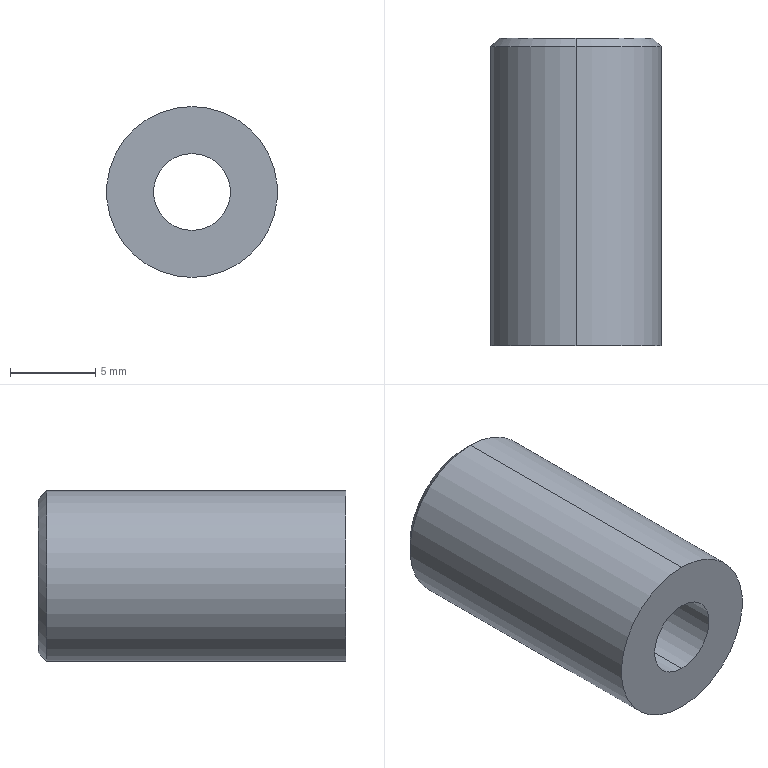Part | SolidWorks | features Chamfer 1, Extrusion 1, HoleWzd 1 | 1 solid | 11 faces | box 10 x 18 x 10 mm | volume 965.582 mm3 | cylinder 6 | plane 3 | cone 2 | commonest cylinder face diameters 4.5 x2 8 x2 10 x2
STEP:
#1=CARTESIAN_POINT('',(0.,18.,4.5));
#2=VERTEX_POINT('',#1);
#3=CARTESIAN_POINT('',(0.,18.,-4.5));
#4=VERTEX_POINT('',#3);
#5=CARTESIAN_POINT('',(0.,18.,0.));
#6=DIRECTION('',(0.,1.,0.));
#7=DIRECTION('',(0.,0.,1.));
#8=AXIS2_PLACEMENT_3D('',#5,#6,#7);
#9=CIRCLE('',#8,4.5);
#10=EDGE_CURVE('',#2,#4,#9,.T.);
#11=ORIENTED_EDGE('',*,*,#10,.F.);
#12=CARTESIAN_POINT('',(0.,17.5,5.));
#13=VERTEX_POINT('',#12);
#14=CARTESIAN_POINT('',(0.,18.,4.5));
#15=DIRECTION('',(0.,-0.7071,0.7071));
#16=VECTOR('',#15,1000.);
#17=LINE('',#14,#16);
#18=EDGE_CURVE('',#2,#13,#17,.T.);
#19=ORIENTED_EDGE('',*,*,#18,.T.);
#20=CARTESIAN_POINT('',(0.,17.5,-5.));
#21=VERTEX_POINT('',#20);
#22=CARTESIAN_POINT('',(0.,17.5,0.));
#23=DIRECTION('',(0.,-1.,0.));
#24=DIRECTION('',(0.,0.,1.));
#25=AXIS2_PLACEMENT_3D('',#22,#23,#24);
#26=CIRCLE('',#25,5.);
#27=EDGE_CURVE('',#21,#13,#26,.T.);
#28=ORIENTED_EDGE('',*,*,#27,.F.);
#29=CARTESIAN_POINT('',(0.,18.,-4.5));
#30=DIRECTION('',(0.,-0.7071,-0.7071));
#31=VECTOR('',#30,1000.);
#32=LINE('',#29,#31);
#33=EDGE_CURVE('',#4,#21,#32,.T.);
#34=ORIENTED_EDGE('',*,*,#33,.F.);
#35=EDGE_LOOP('',(#11,#19,#28,#34));
#36=FACE_OUTER_BOUND('',#35,.T.);
#37=CARTESIAN_POINT('',(0.,18.,0.));
#38=DIRECTION('',(0.,-1.,0.));
#39=DIRECTION('',(0.,0.,-1.));
#40=AXIS2_PLACEMENT_3D('',#37,#38,#39);
#41=CONICAL_SURFACE('',#40,4.5,0.7854);
#42=ADVANCED_FACE('',(#36),#41,.T.);
#43=CARTESIAN_POINT('',(0.,13.4,-4.));
#44=VERTEX_POINT('',#43);
#45=CARTESIAN_POINT('',(0.,13.4,4.));
#46=VERTEX_POINT('',#45);
#47=CARTESIAN_POINT('',(0.,13.4,0.));
#48=DIRECTION('',(0.,1.,0.));
#49=DIRECTION('',(0.,0.,1.));
#50=AXIS2_PLACEMENT_3D('',#47,#48,#49);
#51=CIRCLE('',#50,4.);
#52=EDGE_CURVE('',#44,#46,#51,.T.);
#53=ORIENTED_EDGE('',*,*,#52,.F.);
#54=CARTESIAN_POINT('',(0.,18.,-4.));
#55=VERTEX_POINT('',#54);
#56=CARTESIAN_POINT('',(0.,18.,-4.));
#57=DIRECTION('',(0.,1.,0.));
#58=VECTOR('',#57,1000.);
#59=LINE('',#56,#58);
#60=EDGE_CURVE('',#44,#55,#59,.T.);
#61=ORIENTED_EDGE('',*,*,#60,.T.);
#62=CARTESIAN_POINT('',(0.,18.,4.));
#63=VERTEX_POINT('',#62);
#64=CARTESIAN_POINT('',(0.,18.,0.));
#65=DIRECTION('',(0.,1.,0.));
#66=DIRECTION('',(0.,0.,1.));
#67=AXIS2_PLACEMENT_3D('',#64,#65,#66);
#68=CIRCLE('',#67,4.);
#69=EDGE_CURVE('',#55,#63,#68,.T.);
#70=ORIENTED_EDGE('',*,*,#69,.T.);
#71=CARTESIAN_POINT('',(0.,18.,4.));
#72=DIRECTION('',(0.,1.,0.));
#73=VECTOR('',#72,1000.);
#74=LINE('',#71,#73);
#75=EDGE_CURVE('',#46,#63,#74,.T.);
#76=ORIENTED_EDGE('',*,*,#75,.F.);
#77=EDGE_LOOP('',(#53,#61,#70,#76));
#78=FACE_OUTER_BOUND('',#77,.T.);
#79=CARTESIAN_POINT('',(0.,18.,0.));
#80=DIRECTION('',(0.,1.,0.));
#81=DIRECTION('',(0.,0.,1.));
#82=AXIS2_PLACEMENT_3D('',#79,#80,#81);
#83=CYLINDRICAL_SURFACE('',#82,4.);
#84=ADVANCED_FACE('',(#78),#83,.F.);
#85=CARTESIAN_POINT('',(0.,0.,-2.25));
#86=VERTEX_POINT('',#85);
#87=CARTESIAN_POINT('',(0.,0.,2.25));
#88=VERTEX_POINT('',#87);
#89=CARTESIAN_POINT('',(0.,0.,0.));
#90=DIRECTION('',(0.,1.,0.));
#91=DIRECTION('',(0.,0.,1.));
#92=AXIS2_PLACEMENT_3D('',#89,#90,#91);
#93=CIRCLE('',#92,2.25);
#94=EDGE_CURVE('',#86,#88,#93,.T.);
#95=ORIENTED_EDGE('',*,*,#94,.F.);
#96=CARTESIAN_POINT('',(0.,13.4,-2.25));
#97=VERTEX_POINT('',#96);
#98=CARTESIAN_POINT('',(0.,18.,-2.25));
#99=DIRECTION('',(0.,1.,0.));
#100=VECTOR('',#99,1000.);
#101=LINE('',#98,#100);
#102=EDGE_CURVE('',#86,#97,#101,.T.);
#103=ORIENTED_EDGE('',*,*,#102,.T.);
#104=CARTESIAN_POINT('',(0.,13.4,2.25));
#105=VERTEX_POINT('',#104);
#106=CARTESIAN_POINT('',(0.,13.4,0.));
#107=DIRECTION('',(0.,1.,0.));
#108=DIRECTION('',(0.,0.,1.));
#109=AXIS2_PLACEMENT_3D('',#106,#107,#108);
#110=CIRCLE('',#109,2.25);
#111=EDGE_CURVE('',#97,#105,#110,.T.);
#112=ORIENTED_EDGE('',*,*,#111,.T.);
#113=CARTESIAN_POINT('',(0.,18.,2.25));
#114=DIRECTION('',(0.,1.,0.));
#115=VECTOR('',#114,1000.);
#116=LINE('',#113,#115);
#117=EDGE_CURVE('',#88,#105,#116,.T.);
#118=ORIENTED_EDGE('',*,*,#117,.F.);
#119=EDGE_LOOP('',(#95,#103,#112,#118));
#120=FACE_OUTER_BOUND('',#119,.T.);
#121=CARTESIAN_POINT('',(0.,18.,0.));
#122=DIRECTION('',(0.,1.,0.));
#123=DIRECTION('',(0.,0.,1.));
#124=AXIS2_PLACEMENT_3D('',#121,#122,#123);
#125=CYLINDRICAL_SURFACE('',#124,2.25);
#126=ADVANCED_FACE('',(#120),#125,.F.);
#127=ORIENTED_EDGE('',*,*,#27,.T.);
#128=CARTESIAN_POINT('',(0.,0.,5.));
#129=VERTEX_POINT('',#128);
#130=CARTESIAN_POINT('',(0.,18.,5.));
#131=DIRECTION('',(0.,-1.,0.));
#132=VECTOR('',#131,1000.);
#133=LINE('',#130,#132);
#134=EDGE_CURVE('',#13,#129,#133,.T.);
#135=ORIENTED_EDGE('',*,*,#134,.T.);
#136=CARTESIAN_POINT('',(0.,0.,-5.));
#137=VERTEX_POINT('',#136);
#138=CARTESIAN_POINT('',(0.,0.,0.));
#139=DIRECTION('',(0.,1.,0.));
#140=DIRECTION('',(0.,0.,1.));
#141=AXIS2_PLACEMENT_3D('',#138,#139,#140);
#142=CIRCLE('',#141,5.);
#143=EDGE_CURVE('',#129,#137,#142,.T.);
#144=ORIENTED_EDGE('',*,*,#143,.T.);
#145=CARTESIAN_POINT('',(0.,18.,-5.));
#146=DIRECTION('',(0.,-1.,0.));
#147=VECTOR('',#146,1000.);
#148=LINE('',#145,#147);
#149=EDGE_CURVE('',#21,#137,#148,.T.);
#150=ORIENTED_EDGE('',*,*,#149,.F.);
#151=EDGE_LOOP('',(#127,#135,#144,#150));
#152=FACE_OUTER_BOUND('',#151,.T.);
#153=CARTESIAN_POINT('',(0.,18.,0.));
#154=DIRECTION('',(0.,-1.,0.));
#155=DIRECTION('',(0.,0.,-1.));
#156=AXIS2_PLACEMENT_3D('',#153,#154,#155);
#157=CYLINDRICAL_SURFACE('',#156,5.);
#158=ADVANCED_FACE('',(#152),#157,.T.);
#159=ORIENTED_EDGE('',*,*,#134,.F.);
#160=CARTESIAN_POINT('',(0.,17.5,0.));
#161=DIRECTION('',(0.,-1.,0.));
#162=DIRECTION('',(0.,0.,1.));
#163=AXIS2_PLACEMENT_3D('',#160,#161,#162);
#164=CIRCLE('',#163,5.);
#165=EDGE_CURVE('',#13,#21,#164,.T.);
#166=ORIENTED_EDGE('',*,*,#165,.T.);
#167=ORIENTED_EDGE('',*,*,#149,.T.);
#168=CARTESIAN_POINT('',(0.,0.,0.));
#169=DIRECTION('',(0.,1.,0.));
#170=DIRECTION('',(0.,0.,1.));
#171=AXIS2_PLACEMENT_3D('',#168,#169,#170);
#172=CIRCLE('',#171,5.);
#173=EDGE_CURVE('',#137,#129,#172,.T.);
#174=ORIENTED_EDGE('',*,*,#173,.T.);
#175=EDGE_LOOP('',(#159,#166,#167,#174));
#176=FACE_OUTER_BOUND('',#175,.T.);
#177=CARTESIAN_POINT('',(0.,18.,0.));
#178=DIRECTION('',(0.,-1.,0.));
#179=DIRECTION('',(0.,0.,-1.));
#180=AXIS2_PLACEMENT_3D('',#177,#178,#179);
#181=CYLINDRICAL_SURFACE('',#180,5.);
#182=ADVANCED_FACE('',(#176),#181,.T.);
#183=CARTESIAN_POINT('',(0.,18.,0.));
#184=DIRECTION('',(0.,1.,0.));
#185=DIRECTION('',(0.,0.,1.));
#186=AXIS2_PLACEMENT_3D('',#183,#184,#185);
#187=CIRCLE('',#186,4.5);
#188=EDGE_CURVE('',#4,#2,#187,.T.);
#189=ORIENTED_EDGE('',*,*,#188,.T.);
#190=ORIENTED_EDGE('',*,*,#10,.T.);
#191=EDGE_LOOP('',(#189,#190));
#192=FACE_OUTER_BOUND('',#191,.T.);
#193=CARTESIAN_POINT('',(0.,18.,0.));
#194=DIRECTION('',(0.,1.,0.));
#195=DIRECTION('',(0.,0.,1.));
#196=AXIS2_PLACEMENT_3D('',#193,#194,#195);
#197=CIRCLE('',#196,4.);
#198=EDGE_CURVE('',#63,#55,#197,.T.);
#199=ORIENTED_EDGE('',*,*,#198,.F.);
#200=ORIENTED_EDGE('',*,*,#69,.F.);
#201=EDGE_LOOP('',(#199,#200));
#202=FACE_BOUND('',#201,.T.);
#203=CARTESIAN_POINT('',(0.,18.,0.));
#204=DIRECTION('',(0.,1.,0.));
#205=DIRECTION('',(0.,0.,1.));
#206=AXIS2_PLACEMENT_3D('',#203,#204,#205);
#207=PLANE('',#206);
#208=ADVANCED_FACE('',(#192,#202),#207,.T.);
#209=CARTESIAN_POINT('',(0.,0.,0.));
#210=DIRECTION('',(0.,1.,0.));
#211=DIRECTION('',(0.,0.,1.));
#212=AXIS2_PLACEMENT_3D('',#209,#210,#211);
#213=CIRCLE('',#212,2.25);
#214=EDGE_CURVE('',#88,#86,#213,.T.);
#215=ORIENTED_EDGE('',*,*,#214,.T.);
#216=ORIENTED_EDGE('',*,*,#94,.T.);
#217=EDGE_LOOP('',(#215,#216));
#218=FACE_BOUND('',#217,.T.);
#219=ORIENTED_EDGE('',*,*,#173,.F.);
#220=ORIENTED_EDGE('',*,*,#143,.F.);
#221=EDGE_LOOP('',(#219,#220));
#222=FACE_OUTER_BOUND('',#221,.T.);
#223=CARTESIAN_POINT('',(0.,0.,0.));
#224=DIRECTION('',(0.,1.,0.));
#225=DIRECTION('',(0.,0.,1.));
#226=AXIS2_PLACEMENT_3D('',#223,#224,#225);
#227=PLANE('',#226);
#228=ADVANCED_FACE('',(#218,#222),#227,.F.);
#229=ORIENTED_EDGE('',*,*,#102,.F.);
#230=ORIENTED_EDGE('',*,*,#214,.F.);
#231=ORIENTED_EDGE('',*,*,#117,.T.);
#232=CARTESIAN_POINT('',(0.,13.4,0.));
#233=DIRECTION('',(0.,1.,0.));
#234=DIRECTION('',(0.,0.,1.));
#235=AXIS2_PLACEMENT_3D('',#232,#233,#234);
#236=CIRCLE('',#235,2.25);
#237=EDGE_CURVE('',#105,#97,#236,.T.);
#238=ORIENTED_EDGE('',*,*,#237,.T.);
#239=EDGE_LOOP('',(#229,#230,#231,#238));
#240=FACE_OUTER_BOUND('',#239,.T.);
#241=CARTESIAN_POINT('',(0.,18.,0.));
#242=DIRECTION('',(0.,1.,0.));
#243=DIRECTION('',(0.,0.,1.));
#244=AXIS2_PLACEMENT_3D('',#241,#242,#243);
#245=CYLINDRICAL_SURFACE('',#244,2.25);
#246=ADVANCED_FACE('',(#240),#245,.F.);
#247=ORIENTED_EDGE('',*,*,#237,.F.);
#248=ORIENTED_EDGE('',*,*,#111,.F.);
#249=EDGE_LOOP('',(#247,#248));
#250=FACE_BOUND('',#249,.T.);
#251=CARTESIAN_POINT('',(0.,13.4,0.));
#252=DIRECTION('',(0.,1.,0.));
#253=DIRECTION('',(0.,0.,1.));
#254=AXIS2_PLACEMENT_3D('',#251,#252,#253);
#255=CIRCLE('',#254,4.);
#256=EDGE_CURVE('',#46,#44,#255,.T.);
#257=ORIENTED_EDGE('',*,*,#256,.T.);
#258=ORIENTED_EDGE('',*,*,#52,.T.);
#259=EDGE_LOOP('',(#257,#258));
#260=FACE_OUTER_BOUND('',#259,.T.);
#261=CARTESIAN_POINT('',(2.25,13.4,0.));
#262=DIRECTION('',(0.,-1.,0.));
#263=DIRECTION('',(0.,0.,-1.));
#264=AXIS2_PLACEMENT_3D('',#261,#262,#263);
#265=PLANE('',#264);
#266=ADVANCED_FACE('',(#250,#260),#265,.F.);
#267=ORIENTED_EDGE('',*,*,#60,.F.);
#268=ORIENTED_EDGE('',*,*,#256,.F.);
#269=ORIENTED_EDGE('',*,*,#75,.T.);
#270=ORIENTED_EDGE('',*,*,#198,.T.);
#271=EDGE_LOOP('',(#267,#268,#269,#270));
#272=FACE_OUTER_BOUND('',#271,.T.);
#273=CARTESIAN_POINT('',(0.,18.,0.));
#274=DIRECTION('',(0.,1.,0.));
#275=DIRECTION('',(0.,0.,1.));
#276=AXIS2_PLACEMENT_3D('',#273,#274,#275);
#277=CYLINDRICAL_SURFACE('',#276,4.);
#278=ADVANCED_FACE('',(#272),#277,.F.);
#279=ORIENTED_EDGE('',*,*,#18,.F.);
#280=ORIENTED_EDGE('',*,*,#188,.F.);
#281=ORIENTED_EDGE('',*,*,#33,.T.);
#282=ORIENTED_EDGE('',*,*,#165,.F.);
#283=EDGE_LOOP('',(#279,#280,#281,#282));
#284=FACE_OUTER_BOUND('',#283,.T.);
#285=CARTESIAN_POINT('',(0.,18.,0.));
#286=DIRECTION('',(0.,-1.,0.));
#287=DIRECTION('',(0.,0.,-1.));
#288=AXIS2_PLACEMENT_3D('',#285,#286,#287);
#289=CONICAL_SURFACE('',#288,4.5,0.7854);
#290=ADVANCED_FACE('',(#284),#289,.T.);
#291=CLOSED_SHELL('',(#42,#84,#126,#158,#182,#208,#228,#246,#266,#278,#290));
#292=MANIFOLD_SOLID_BREP('',#291);
#293=CARTESIAN_POINT('',(0.,0.,0.));
#294=DIRECTION('',(0.,0.,1.));
#295=DIRECTION('',(1.,0.,0.));
#296=AXIS2_PLACEMENT_3D('',#293,#294,#295);
#297=(LENGTH_UNIT()NAMED_UNIT(*)SI_UNIT(.MILLI.,.METRE.));
#298=UNCERTAINTY_MEASURE_WITH_UNIT(LENGTH_MEASURE(0.00001),#297,'','');
#299=(NAMED_UNIT(*)PLANE_ANGLE_UNIT()SI_UNIT($,.RADIAN.));
#300=(NAMED_UNIT(*)SI_UNIT($,.STERADIAN.)SOLID_ANGLE_UNIT());
#301=(GEOMETRIC_REPRESENTATION_CONTEXT(3)GLOBAL_UNCERTAINTY_ASSIGNED_CONTEXT((#298))GLOBAL_UNIT_ASSIGNED_CONTEXT((#297,#299,#300))REPRESENTATION_CONTEXT('',''));
#302=ADVANCED_BREP_SHAPE_REPRESENTATION('',(#292,#296),#301);